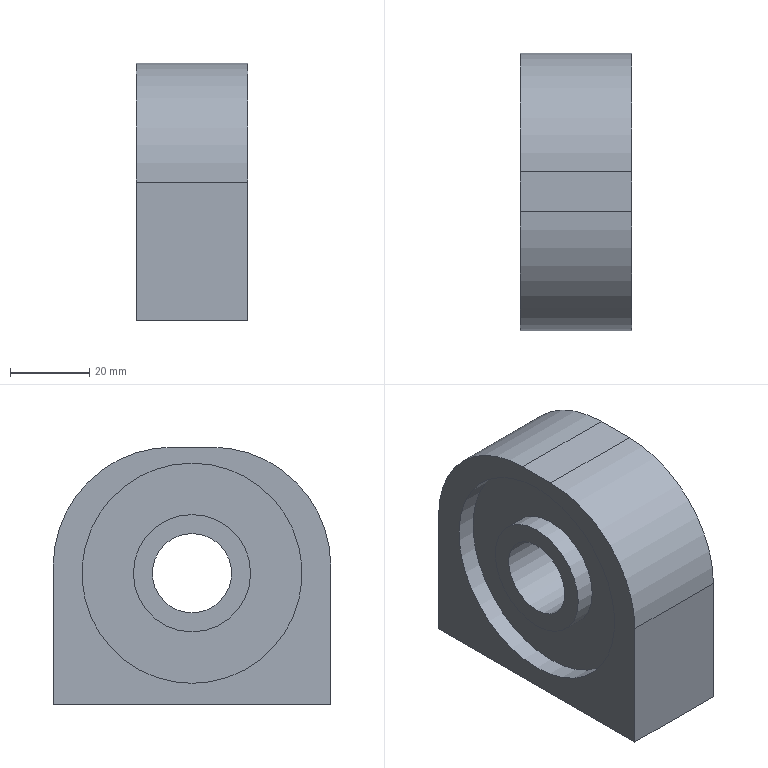Part | STEP file | Housing | 1 solid | 21 faces | box 28 x 70 x 65 mm | volume 87955 mm3 | plane 12 | cylinder 9 | commonest cylinder face diameters 8 x2 29.588 x2 55.503 x2 60 x2 20 x1
STEP:
#1=CARTESIAN_POINT('',(0.,0.,0.));
#2=DIRECTION('',(0.,0.,1.));
#3=DIRECTION('',(1.,0.,0.));
#4=AXIS2_PLACEMENT_3D('',#1,#2,#3);
#5=CARTESIAN_POINT('',(5.,-35.,47.994));
#6=VERTEX_POINT('',#5);
#7=CARTESIAN_POINT('',(5.,-35.,33.2));
#8=DIRECTION('',(-1.,0.,0.));
#9=DIRECTION('',(0.,0.,-1.));
#10=AXIS2_PLACEMENT_3D('',#7,#8,#9);
#11=CIRCLE('',#10,14.794);
#12=CARTESIAN_POINT('',(0.,-35.,33.2));
#13=DIRECTION('',(1.,0.,0.));
#14=DIRECTION('',(0.,0.,-1.));
#15=AXIS2_PLACEMENT_3D('',#12,#13,#14);
#16=CYLINDRICAL_SURFACE('',#15,14.794);
#17=CARTESIAN_POINT('',(12.566,5.));
#18=DIRECTION('',(-1.,0.));
#19=VECTOR('',#18,1.);
#20=LINE('',#17,#19);
#21=(GEOMETRIC_REPRESENTATION_CONTEXT(2)PARAMETRIC_REPRESENTATION_CONTEXT()REPRESENTATION_CONTEXT('',''));
#22=DEFINITIONAL_REPRESENTATION('',(#20),#21);
#23=PCURVE('',#16,#22);
#24=CARTESIAN_POINT('',(5.,-35.,33.2));
#25=DIRECTION('',(-1.,0.,0.));
#26=DIRECTION('',(0.,0.,1.));
#27=AXIS2_PLACEMENT_3D('',#24,#25,#26);
#28=PLANE('',#27);
#29=CARTESIAN_POINT('',(0.,0.));
#30=DIRECTION('',(-1.,0.));
#31=AXIS2_PLACEMENT_2D('',#29,#30);
#32=CIRCLE('',#31,14.794);
#33=(GEOMETRIC_REPRESENTATION_CONTEXT(2)PARAMETRIC_REPRESENTATION_CONTEXT()REPRESENTATION_CONTEXT('',''));
#34=DEFINITIONAL_REPRESENTATION('',(#32),#33);
#35=PCURVE('',#28,#34);
#36=SURFACE_CURVE('',#11,(#23,#35),.PCURVE_S1.);
#37=EDGE_CURVE('',#6,#6,#36,.T.);
#38=ORIENTED_EDGE('',*,*,#37,.T.);
#39=CARTESIAN_POINT('',(0.,-35.,47.994));
#40=VERTEX_POINT('',#39);
#41=CARTESIAN_POINT('',(0.,-35.,47.994));
#42=CARTESIAN_POINT('',(5.,-35.,47.994));
#43=B_SPLINE_CURVE_WITH_KNOTS('',1,(#41,#42),.UNSPECIFIED.,.F.,.F.,(2,2),(0.,5.),.PIECEWISE_BEZIER_KNOTS.);
#44=CARTESIAN_POINT('',(3.142,0.));
#45=DIRECTION('',(0.,1.));
#46=VECTOR('',#45,1.);
#47=LINE('',#44,#46);
#48=(GEOMETRIC_REPRESENTATION_CONTEXT(2)PARAMETRIC_REPRESENTATION_CONTEXT()REPRESENTATION_CONTEXT('',''));
#49=DEFINITIONAL_REPRESENTATION('',(#47),#48);
#50=PCURVE('',#16,#49);
#51=CARTESIAN_POINT('',(9.425,0.));
#52=DIRECTION('',(0.,1.));
#53=VECTOR('',#52,1.);
#54=LINE('',#51,#53);
#55=(GEOMETRIC_REPRESENTATION_CONTEXT(2)PARAMETRIC_REPRESENTATION_CONTEXT()REPRESENTATION_CONTEXT('',''));
#56=DEFINITIONAL_REPRESENTATION('',(#54),#55);
#57=PCURVE('',#16,#56);
#58=SEAM_CURVE('',#43,(#50,#57),.PCURVE_S1.);
#59=EDGE_CURVE('',#40,#6,#58,.T.);
#60=ORIENTED_EDGE('',*,*,#59,.F.);
#61=CARTESIAN_POINT('',(0.,-35.,33.2));
#62=DIRECTION('',(-1.,0.,0.));
#63=DIRECTION('',(0.,0.,-1.));
#64=AXIS2_PLACEMENT_3D('',#61,#62,#63);
#65=CIRCLE('',#64,14.794);
#66=CARTESIAN_POINT('',(12.566,0.));
#67=DIRECTION('',(-1.,0.));
#68=VECTOR('',#67,1.);
#69=LINE('',#66,#68);
#70=(GEOMETRIC_REPRESENTATION_CONTEXT(2)PARAMETRIC_REPRESENTATION_CONTEXT()REPRESENTATION_CONTEXT('',''));
#71=DEFINITIONAL_REPRESENTATION('',(#69),#70);
#72=PCURVE('',#16,#71);
#73=CARTESIAN_POINT('',(0.,0.,0.));
#74=DIRECTION('',(-1.,0.,0.));
#75=DIRECTION('',(0.,-1.,0.));
#76=AXIS2_PLACEMENT_3D('',#73,#74,#75);
#77=PLANE('',#76);
#78=CARTESIAN_POINT('',(35.,33.2));
#79=DIRECTION('',(0.,-1.));
#80=AXIS2_PLACEMENT_2D('',#78,#79);
#81=CIRCLE('',#80,14.794);
#82=(GEOMETRIC_REPRESENTATION_CONTEXT(2)PARAMETRIC_REPRESENTATION_CONTEXT()REPRESENTATION_CONTEXT('',''));
#83=DEFINITIONAL_REPRESENTATION('',(#81),#82);
#84=PCURVE('',#77,#83);
#85=SURFACE_CURVE('',#65,(#72,#84),.PCURVE_S1.);
#86=EDGE_CURVE('',#40,#40,#85,.T.);
#87=ORIENTED_EDGE('',*,*,#86,.F.);
#88=ORIENTED_EDGE('',*,*,#59,.T.);
#89=EDGE_LOOP('',(#38,#60,#87,#88));
#90=FACE_BOUND('',#89,.T.);
#91=ADVANCED_FACE('',(#90),#16,.T.);
#92=CARTESIAN_POINT('',(5.,-35.,60.951));
#93=VERTEX_POINT('',#92);
#94=CARTESIAN_POINT('',(5.,-35.,33.2));
#95=DIRECTION('',(1.,0.,0.));
#96=DIRECTION('',(0.,0.,-1.));
#97=AXIS2_PLACEMENT_3D('',#94,#95,#96);
#98=CIRCLE('',#97,27.751);
#99=CARTESIAN_POINT('',(0.,-35.,33.2));
#100=DIRECTION('',(1.,0.,0.));
#101=DIRECTION('',(0.,0.,-1.));
#102=AXIS2_PLACEMENT_3D('',#99,#100,#101);
#103=CYLINDRICAL_SURFACE('',#102,27.751);
#104=CARTESIAN_POINT('',(0.,5.));
#105=DIRECTION('',(1.,0.));
#106=VECTOR('',#105,1.);
#107=LINE('',#104,#106);
#108=(GEOMETRIC_REPRESENTATION_CONTEXT(2)PARAMETRIC_REPRESENTATION_CONTEXT()REPRESENTATION_CONTEXT('',''));
#109=DEFINITIONAL_REPRESENTATION('',(#107),#108);
#110=PCURVE('',#103,#109);
#111=CARTESIAN_POINT('',(-27.751,0.));
#112=CARTESIAN_POINT('',(-27.751,48.067));
#113=CARTESIAN_POINT('',(13.876,24.033));
#114=CARTESIAN_POINT('',(55.503,0.));
#115=CARTESIAN_POINT('',(13.876,-24.033));
#116=CARTESIAN_POINT('',(-27.751,-48.067));
#117=CARTESIAN_POINT('',(-27.751,0.));
#118=(BOUNDED_CURVE()B_SPLINE_CURVE(2,(#111,#112,#113,#114,#115,#116,#117),.UNSPECIFIED.,.T.,.F.)B_SPLINE_CURVE_WITH_KNOTS((1,2,2,2,2,1),(-2.094,0.,2.094,4.189,6.283,8.378),.UNSPECIFIED.)CURVE()GEOMETRIC_REPRESENTATION_ITEM()RATIONAL_B_SPLINE_CURVE((1.,0.5,1.,0.5,1.,0.5,1.))REPRESENTATION_ITEM(''));
#119=(GEOMETRIC_REPRESENTATION_CONTEXT(2)PARAMETRIC_REPRESENTATION_CONTEXT()REPRESENTATION_CONTEXT('',''));
#120=DEFINITIONAL_REPRESENTATION('',(#118),#119);
#121=PCURVE('',#28,#120);
#122=SURFACE_CURVE('',#98,(#110,#121),.PCURVE_S1.);
#123=EDGE_CURVE('',#93,#93,#122,.T.);
#124=ORIENTED_EDGE('',*,*,#123,.F.);
#125=CARTESIAN_POINT('',(0.,-35.,60.951));
#126=VERTEX_POINT('',#125);
#127=CARTESIAN_POINT('',(0.,-35.,60.951));
#128=CARTESIAN_POINT('',(5.,-35.,60.951));
#129=B_SPLINE_CURVE_WITH_KNOTS('',1,(#127,#128),.UNSPECIFIED.,.F.,.F.,(2,2),(0.,5.),.PIECEWISE_BEZIER_KNOTS.);
#130=CARTESIAN_POINT('',(3.142,0.));
#131=DIRECTION('',(0.,1.));
#132=VECTOR('',#131,1.);
#133=LINE('',#130,#132);
#134=(GEOMETRIC_REPRESENTATION_CONTEXT(2)PARAMETRIC_REPRESENTATION_CONTEXT()REPRESENTATION_CONTEXT('',''));
#135=DEFINITIONAL_REPRESENTATION('',(#133),#134);
#136=PCURVE('',#103,#135);
#137=CARTESIAN_POINT('',(9.425,0.));
#138=DIRECTION('',(0.,1.));
#139=VECTOR('',#138,1.);
#140=LINE('',#137,#139);
#141=(GEOMETRIC_REPRESENTATION_CONTEXT(2)PARAMETRIC_REPRESENTATION_CONTEXT()REPRESENTATION_CONTEXT('',''));
#142=DEFINITIONAL_REPRESENTATION('',(#140),#141);
#143=PCURVE('',#103,#142);
#144=SEAM_CURVE('',#129,(#136,#143),.PCURVE_S1.);
#145=EDGE_CURVE('',#126,#93,#144,.T.);
#146=ORIENTED_EDGE('',*,*,#145,.F.);
#147=CARTESIAN_POINT('',(0.,-35.,33.2));
#148=DIRECTION('',(1.,0.,0.));
#149=DIRECTION('',(0.,0.,-1.));
#150=AXIS2_PLACEMENT_3D('',#147,#148,#149);
#151=CIRCLE('',#150,27.751);
#152=CARTESIAN_POINT('',(0.,0.));
#153=DIRECTION('',(1.,0.));
#154=VECTOR('',#153,1.);
#155=LINE('',#152,#154);
#156=(GEOMETRIC_REPRESENTATION_CONTEXT(2)PARAMETRIC_REPRESENTATION_CONTEXT()REPRESENTATION_CONTEXT('',''));
#157=DEFINITIONAL_REPRESENTATION('',(#155),#156);
#158=PCURVE('',#103,#157);
#159=CARTESIAN_POINT('',(0.,0.,0.));
#160=DIRECTION('',(-1.,0.,0.));
#161=DIRECTION('',(0.,-1.,0.));
#162=AXIS2_PLACEMENT_3D('',#159,#160,#161);
#163=PLANE('',#162);
#164=CARTESIAN_POINT('',(35.,5.449));
#165=CARTESIAN_POINT('',(-13.067,5.449));
#166=CARTESIAN_POINT('',(10.967,47.076));
#167=CARTESIAN_POINT('',(35.,88.703));
#168=CARTESIAN_POINT('',(59.033,47.076));
#169=CARTESIAN_POINT('',(83.067,5.449));
#170=CARTESIAN_POINT('',(35.,5.449));
#171=(BOUNDED_CURVE()B_SPLINE_CURVE(2,(#164,#165,#166,#167,#168,#169,#170),.UNSPECIFIED.,.T.,.F.)B_SPLINE_CURVE_WITH_KNOTS((1,2,2,2,2,1),(-2.094,0.,2.094,4.189,6.283,8.378),.UNSPECIFIED.)CURVE()GEOMETRIC_REPRESENTATION_ITEM()RATIONAL_B_SPLINE_CURVE((1.,0.5,1.,0.5,1.,0.5,1.))REPRESENTATION_ITEM(''));
#172=(GEOMETRIC_REPRESENTATION_CONTEXT(2)PARAMETRIC_REPRESENTATION_CONTEXT()REPRESENTATION_CONTEXT('',''));
#173=DEFINITIONAL_REPRESENTATION('',(#171),#172);
#174=PCURVE('',#163,#173);
#175=SURFACE_CURVE('',#151,(#158,#174),.PCURVE_S1.);
#176=EDGE_CURVE('',#126,#126,#175,.T.);
#177=ORIENTED_EDGE('',*,*,#176,.T.);
#178=ORIENTED_EDGE('',*,*,#145,.T.);
#179=EDGE_LOOP('',(#124,#146,#177,#178));
#180=FACE_BOUND('',#179,.F.);
#181=ADVANCED_FACE('',(#180),#103,.F.);
#182=ORIENTED_EDGE('',*,*,#123,.F.);
#183=EDGE_LOOP('',(#182));
#184=FACE_BOUND('',#183,.T.);
#185=ORIENTED_EDGE('',*,*,#37,.F.);
#186=EDGE_LOOP('',(#185));
#187=FACE_BOUND('',#186,.T.);
#188=ADVANCED_FACE('',(#184,#187),#28,.T.);
#189=CARTESIAN_POINT('',(0.,-40.,65.));
#190=VERTEX_POINT('',#189);
#191=CARTESIAN_POINT('',(0.,-70.,35.));
#192=VERTEX_POINT('',#191);
#193=CARTESIAN_POINT('',(0.,-40.,35.));
#194=DIRECTION('',(1.,0.,0.));
#195=DIRECTION('',(0.,-0.7071,0.7071));
#196=AXIS2_PLACEMENT_3D('',#193,#194,#195);
#197=CIRCLE('',#196,30.);
#198=CARTESIAN_POINT('',(61.213,56.213));
#199=CARTESIAN_POINT('',(97.956,19.471));
#200=CARTESIAN_POINT('',(47.765,6.022));
#201=CARTESIAN_POINT('',(-2.426,-7.426));
#202=CARTESIAN_POINT('',(11.022,42.765));
#203=CARTESIAN_POINT('',(24.471,92.956));
#204=CARTESIAN_POINT('',(61.213,56.213));
#205=(BOUNDED_CURVE()B_SPLINE_CURVE(2,(#198,#199,#200,#201,#202,#203,#204),.UNSPECIFIED.,.T.,.F.)B_SPLINE_CURVE_WITH_KNOTS((1,2,2,2,2,1),(-2.094,0.,2.094,4.189,6.283,8.378),.UNSPECIFIED.)CURVE()GEOMETRIC_REPRESENTATION_ITEM()RATIONAL_B_SPLINE_CURVE((1.,0.5,1.,0.5,1.,0.5,1.))REPRESENTATION_ITEM(''));
#206=(GEOMETRIC_REPRESENTATION_CONTEXT(2)PARAMETRIC_REPRESENTATION_CONTEXT()REPRESENTATION_CONTEXT('',''));
#207=DEFINITIONAL_REPRESENTATION('',(#205),#206);
#208=PCURVE('',#163,#207);
#209=CARTESIAN_POINT('',(7.,-40.,35.));
#210=DIRECTION('',(1.,0.,0.));
#211=DIRECTION('',(0.,-0.7071,0.7071));
#212=AXIS2_PLACEMENT_3D('',#209,#210,#211);
#213=CYLINDRICAL_SURFACE('',#212,30.);
#214=CARTESIAN_POINT('',(-6.283,-7.));
#215=DIRECTION('',(1.,0.));
#216=VECTOR('',#215,1.);
#217=LINE('',#214,#216);
#218=(GEOMETRIC_REPRESENTATION_CONTEXT(2)PARAMETRIC_REPRESENTATION_CONTEXT()REPRESENTATION_CONTEXT('',''));
#219=DEFINITIONAL_REPRESENTATION('',(#217),#218);
#220=PCURVE('',#213,#219);
#221=SURFACE_CURVE('',#197,(#208,#220),.PCURVE_S1.);
#222=EDGE_CURVE('',#190,#192,#221,.T.);
#223=ORIENTED_EDGE('',*,*,#222,.F.);
#224=CARTESIAN_POINT('',(0.,-30.,65.));
#225=VERTEX_POINT('',#224);
#226=CARTESIAN_POINT('',(0.,-70.,65.));
#227=DIRECTION('',(0.,-1.,0.));
#228=VECTOR('',#227,1.);
#229=LINE('',#226,#228);
#230=CARTESIAN_POINT('',(70.,65.));
#231=DIRECTION('',(1.,0.));
#232=VECTOR('',#231,1.);
#233=LINE('',#230,#232);
#234=(GEOMETRIC_REPRESENTATION_CONTEXT(2)PARAMETRIC_REPRESENTATION_CONTEXT()REPRESENTATION_CONTEXT('',''));
#235=DEFINITIONAL_REPRESENTATION('',(#233),#234);
#236=PCURVE('',#163,#235);
#237=CARTESIAN_POINT('',(14.,-35.,65.));
#238=DIRECTION('',(0.,0.,1.));
#239=DIRECTION('',(1.,0.,0.));
#240=AXIS2_PLACEMENT_3D('',#237,#238,#239);
#241=PLANE('',#240);
#242=CARTESIAN_POINT('',(-14.,-35.));
#243=DIRECTION('',(0.,-1.));
#244=VECTOR('',#243,1.);
#245=LINE('',#242,#244);
#246=(GEOMETRIC_REPRESENTATION_CONTEXT(2)PARAMETRIC_REPRESENTATION_CONTEXT()REPRESENTATION_CONTEXT('',''));
#247=DEFINITIONAL_REPRESENTATION('',(#245),#246);
#248=PCURVE('',#241,#247);
#249=SURFACE_CURVE('',#229,(#236,#248),.PCURVE_S1.);
#250=EDGE_CURVE('',#225,#190,#249,.T.);
#251=ORIENTED_EDGE('',*,*,#250,.F.);
#252=CARTESIAN_POINT('',(0.,0.,35.));
#253=VERTEX_POINT('',#252);
#254=CARTESIAN_POINT('',(0.,-30.,35.));
#255=DIRECTION('',(1.,0.,0.));
#256=DIRECTION('',(0.,0.7071,0.7071));
#257=AXIS2_PLACEMENT_3D('',#254,#255,#256);
#258=CIRCLE('',#257,30.);
#259=CARTESIAN_POINT('',(8.787,56.213));
#260=CARTESIAN_POINT('',(45.529,92.956));
#261=CARTESIAN_POINT('',(58.978,42.765));
#262=CARTESIAN_POINT('',(72.426,-7.426));
#263=CARTESIAN_POINT('',(22.235,6.022));
#264=CARTESIAN_POINT('',(-27.956,19.471));
#265=CARTESIAN_POINT('',(8.787,56.213));
#266=(BOUNDED_CURVE()B_SPLINE_CURVE(2,(#259,#260,#261,#262,#263,#264,#265),.UNSPECIFIED.,.T.,.F.)B_SPLINE_CURVE_WITH_KNOTS((1,2,2,2,2,1),(-2.094,0.,2.094,4.189,6.283,8.378),.UNSPECIFIED.)CURVE()GEOMETRIC_REPRESENTATION_ITEM()RATIONAL_B_SPLINE_CURVE((1.,0.5,1.,0.5,1.,0.5,1.))REPRESENTATION_ITEM(''));
#267=(GEOMETRIC_REPRESENTATION_CONTEXT(2)PARAMETRIC_REPRESENTATION_CONTEXT()REPRESENTATION_CONTEXT('',''));
#268=DEFINITIONAL_REPRESENTATION('',(#266),#267);
#269=PCURVE('',#163,#268);
#270=CARTESIAN_POINT('',(21.,-30.,35.));
#271=DIRECTION('',(-1.,0.,0.));
#272=DIRECTION('',(0.,0.7071,0.7071));
#273=AXIS2_PLACEMENT_3D('',#270,#271,#272);
#274=CYLINDRICAL_SURFACE('',#273,30.);
#275=CARTESIAN_POINT('',(12.566,21.));
#276=DIRECTION('',(-1.,0.));
#277=VECTOR('',#276,1.);
#278=LINE('',#275,#277);
#279=(GEOMETRIC_REPRESENTATION_CONTEXT(2)PARAMETRIC_REPRESENTATION_CONTEXT()REPRESENTATION_CONTEXT('',''));
#280=DEFINITIONAL_REPRESENTATION('',(#278),#279);
#281=PCURVE('',#274,#280);
#282=SURFACE_CURVE('',#258,(#269,#281),.PCURVE_S1.);
#283=EDGE_CURVE('',#253,#225,#282,.T.);
#284=ORIENTED_EDGE('',*,*,#283,.F.);
#285=CARTESIAN_POINT('',(0.,0.,0.));
#286=VERTEX_POINT('',#285);
#287=CARTESIAN_POINT('',(0.,0.,0.));
#288=DIRECTION('',(0.,0.,1.));
#289=VECTOR('',#288,1.);
#290=LINE('',#287,#289);
#291=CARTESIAN_POINT('',(0.,0.));
#292=DIRECTION('',(0.,1.));
#293=VECTOR('',#292,1.);
#294=LINE('',#291,#293);
#295=(GEOMETRIC_REPRESENTATION_CONTEXT(2)PARAMETRIC_REPRESENTATION_CONTEXT()REPRESENTATION_CONTEXT('',''));
#296=DEFINITIONAL_REPRESENTATION('',(#294),#295);
#297=PCURVE('',#163,#296);
#298=CARTESIAN_POINT('',(28.,0.,0.));
#299=DIRECTION('',(0.,1.,0.));
#300=DIRECTION('',(-1.,0.,0.));
#301=AXIS2_PLACEMENT_3D('',#298,#299,#300);
#302=PLANE('',#301);
#303=CARTESIAN_POINT('',(28.,0.));
#304=DIRECTION('',(0.,1.));
#305=VECTOR('',#304,1.);
#306=LINE('',#303,#305);
#307=(GEOMETRIC_REPRESENTATION_CONTEXT(2)PARAMETRIC_REPRESENTATION_CONTEXT()REPRESENTATION_CONTEXT('',''));
#308=DEFINITIONAL_REPRESENTATION('',(#306),#307);
#309=PCURVE('',#302,#308);
#310=SURFACE_CURVE('',#290,(#297,#309),.PCURVE_S1.);
#311=EDGE_CURVE('',#286,#253,#310,.T.);
#312=ORIENTED_EDGE('',*,*,#311,.F.);
#313=CARTESIAN_POINT('',(0.,-70.,0.));
#314=VERTEX_POINT('',#313);
#315=CARTESIAN_POINT('',(0.,-70.,0.));
#316=DIRECTION('',(0.,1.,0.));
#317=VECTOR('',#316,1.);
#318=LINE('',#315,#317);
#319=CARTESIAN_POINT('',(70.,0.));
#320=DIRECTION('',(-1.,0.));
#321=VECTOR('',#320,1.);
#322=LINE('',#319,#321);
#323=(GEOMETRIC_REPRESENTATION_CONTEXT(2)PARAMETRIC_REPRESENTATION_CONTEXT()REPRESENTATION_CONTEXT('',''));
#324=DEFINITIONAL_REPRESENTATION('',(#322),#323);
#325=PCURVE('',#163,#324);
#326=CARTESIAN_POINT('',(14.,-35.,0.));
#327=DIRECTION('',(0.,0.,1.));
#328=DIRECTION('',(1.,0.,0.));
#329=AXIS2_PLACEMENT_3D('',#326,#327,#328);
#330=PLANE('',#329);
#331=CARTESIAN_POINT('',(-14.,-35.));
#332=DIRECTION('',(0.,1.));
#333=VECTOR('',#332,1.);
#334=LINE('',#331,#333);
#335=(GEOMETRIC_REPRESENTATION_CONTEXT(2)PARAMETRIC_REPRESENTATION_CONTEXT()REPRESENTATION_CONTEXT('',''));
#336=DEFINITIONAL_REPRESENTATION('',(#334),#335);
#337=PCURVE('',#330,#336);
#338=SURFACE_CURVE('',#318,(#325,#337),.PCURVE_S1.);
#339=EDGE_CURVE('',#314,#286,#338,.T.);
#340=ORIENTED_EDGE('',*,*,#339,.F.);
#341=CARTESIAN_POINT('',(0.,-70.,0.));
#342=DIRECTION('',(0.,0.,1.));
#343=VECTOR('',#342,1.);
#344=LINE('',#341,#343);
#345=CARTESIAN_POINT('',(70.,0.));
#346=DIRECTION('',(0.,1.));
#347=VECTOR('',#346,1.);
#348=LINE('',#345,#347);
#349=(GEOMETRIC_REPRESENTATION_CONTEXT(2)PARAMETRIC_REPRESENTATION_CONTEXT()REPRESENTATION_CONTEXT('',''));
#350=DEFINITIONAL_REPRESENTATION('',(#348),#349);
#351=PCURVE('',#163,#350);
#352=CARTESIAN_POINT('',(0.,-70.,0.));
#353=DIRECTION('',(0.,-1.,0.));
#354=DIRECTION('',(1.,0.,0.));
#355=AXIS2_PLACEMENT_3D('',#352,#353,#354);
#356=PLANE('',#355);
#357=CARTESIAN_POINT('',(0.,0.));
#358=DIRECTION('',(0.,1.));
#359=VECTOR('',#358,1.);
#360=LINE('',#357,#359);
#361=(GEOMETRIC_REPRESENTATION_CONTEXT(2)PARAMETRIC_REPRESENTATION_CONTEXT()REPRESENTATION_CONTEXT('',''));
#362=DEFINITIONAL_REPRESENTATION('',(#360),#361);
#363=PCURVE('',#356,#362);
#364=SURFACE_CURVE('',#344,(#351,#363),.PCURVE_S1.);
#365=EDGE_CURVE('',#314,#192,#364,.T.);
#366=ORIENTED_EDGE('',*,*,#365,.T.);
#367=EDGE_LOOP('',(#223,#251,#284,#312,#340,#366));
#368=FACE_BOUND('',#367,.T.);
#369=ORIENTED_EDGE('',*,*,#176,.T.);
#370=EDGE_LOOP('',(#369));
#371=FACE_BOUND('',#370,.T.);
#372=ADVANCED_FACE('',(#368,#371),#163,.T.);
#373=CARTESIAN_POINT('',(23.,-35.,18.406));
#374=VERTEX_POINT('',#373);
#375=CARTESIAN_POINT('',(23.,-35.,33.2));
#376=DIRECTION('',(1.,0.,0.));
#377=DIRECTION('',(0.,0.,1.));
#378=AXIS2_PLACEMENT_3D('',#375,#376,#377);
#379=CIRCLE('',#378,14.794);
#380=CARTESIAN_POINT('',(28.,-35.,33.2));
#381=DIRECTION('',(-1.,0.,0.));
#382=DIRECTION('',(0.,0.,1.));
#383=AXIS2_PLACEMENT_3D('',#380,#381,#382);
#384=CYLINDRICAL_SURFACE('',#383,14.794);
#385=CARTESIAN_POINT('',(12.566,5.));
#386=DIRECTION('',(-1.,0.));
#387=VECTOR('',#386,1.);
#388=LINE('',#385,#387);
#389=(GEOMETRIC_REPRESENTATION_CONTEXT(2)PARAMETRIC_REPRESENTATION_CONTEXT()REPRESENTATION_CONTEXT('',''));
#390=DEFINITIONAL_REPRESENTATION('',(#388),#389);
#391=PCURVE('',#384,#390);
#392=CARTESIAN_POINT('',(23.,-35.,33.2));
#393=DIRECTION('',(-1.,0.,0.));
#394=DIRECTION('',(0.,0.,1.));
#395=AXIS2_PLACEMENT_3D('',#392,#393,#394);
#396=PLANE('',#395);
#397=CARTESIAN_POINT('',(14.794,0.));
#398=CARTESIAN_POINT('',(14.794,-25.624));
#399=CARTESIAN_POINT('',(-7.397,-12.812));
#400=CARTESIAN_POINT('',(-29.588,0.));
#401=CARTESIAN_POINT('',(-7.397,12.812));
#402=CARTESIAN_POINT('',(14.794,25.624));
#403=CARTESIAN_POINT('',(14.794,0.));
#404=(BOUNDED_CURVE()B_SPLINE_CURVE(2,(#397,#398,#399,#400,#401,#402,#403),.UNSPECIFIED.,.T.,.F.)B_SPLINE_CURVE_WITH_KNOTS((1,2,2,2,2,1),(-2.094,0.,2.094,4.189,6.283,8.378),.UNSPECIFIED.)CURVE()GEOMETRIC_REPRESENTATION_ITEM()RATIONAL_B_SPLINE_CURVE((1.,0.5,1.,0.5,1.,0.5,1.))REPRESENTATION_ITEM(''));
#405=(GEOMETRIC_REPRESENTATION_CONTEXT(2)PARAMETRIC_REPRESENTATION_CONTEXT()REPRESENTATION_CONTEXT('',''));
#406=DEFINITIONAL_REPRESENTATION('',(#404),#405);
#407=PCURVE('',#396,#406);
#408=SURFACE_CURVE('',#379,(#391,#407),.PCURVE_S1.);
#409=EDGE_CURVE('',#374,#374,#408,.T.);
#410=ORIENTED_EDGE('',*,*,#409,.T.);
#411=CARTESIAN_POINT('',(28.,-35.,18.406));
#412=VERTEX_POINT('',#411);
#413=CARTESIAN_POINT('',(28.,-35.,18.406));
#414=CARTESIAN_POINT('',(23.,-35.,18.406));
#415=B_SPLINE_CURVE_WITH_KNOTS('',1,(#413,#414),.UNSPECIFIED.,.F.,.F.,(2,2),(0.,5.),.PIECEWISE_BEZIER_KNOTS.);
#416=CARTESIAN_POINT('',(3.142,0.));
#417=DIRECTION('',(0.,1.));
#418=VECTOR('',#417,1.);
#419=LINE('',#416,#418);
#420=(GEOMETRIC_REPRESENTATION_CONTEXT(2)PARAMETRIC_REPRESENTATION_CONTEXT()REPRESENTATION_CONTEXT('',''));
#421=DEFINITIONAL_REPRESENTATION('',(#419),#420);
#422=PCURVE('',#384,#421);
#423=CARTESIAN_POINT('',(9.425,0.));
#424=DIRECTION('',(0.,1.));
#425=VECTOR('',#424,1.);
#426=LINE('',#423,#425);
#427=(GEOMETRIC_REPRESENTATION_CONTEXT(2)PARAMETRIC_REPRESENTATION_CONTEXT()REPRESENTATION_CONTEXT('',''));
#428=DEFINITIONAL_REPRESENTATION('',(#426),#427);
#429=PCURVE('',#384,#428);
#430=SEAM_CURVE('',#415,(#422,#429),.PCURVE_S1.);
#431=EDGE_CURVE('',#412,#374,#430,.T.);
#432=ORIENTED_EDGE('',*,*,#431,.F.);
#433=CARTESIAN_POINT('',(28.,-35.,33.2));
#434=DIRECTION('',(1.,0.,0.));
#435=DIRECTION('',(0.,0.,1.));
#436=AXIS2_PLACEMENT_3D('',#433,#434,#435);
#437=CIRCLE('',#436,14.794);
#438=CARTESIAN_POINT('',(12.566,0.));
#439=DIRECTION('',(-1.,0.));
#440=VECTOR('',#439,1.);
#441=LINE('',#438,#440);
#442=(GEOMETRIC_REPRESENTATION_CONTEXT(2)PARAMETRIC_REPRESENTATION_CONTEXT()REPRESENTATION_CONTEXT('',''));
#443=DEFINITIONAL_REPRESENTATION('',(#441),#442);
#444=PCURVE('',#384,#443);
#445=CARTESIAN_POINT('',(28.,-70.,0.));
#446=DIRECTION('',(1.,0.,0.));
#447=DIRECTION('',(0.,1.,0.));
#448=AXIS2_PLACEMENT_3D('',#445,#446,#447);
#449=PLANE('',#448);
#450=CARTESIAN_POINT('',(35.,33.2));
#451=DIRECTION('',(0.,1.));
#452=AXIS2_PLACEMENT_2D('',#450,#451);
#453=CIRCLE('',#452,14.794);
#454=(GEOMETRIC_REPRESENTATION_CONTEXT(2)PARAMETRIC_REPRESENTATION_CONTEXT()REPRESENTATION_CONTEXT('',''));
#455=DEFINITIONAL_REPRESENTATION('',(#453),#454);
#456=PCURVE('',#449,#455);
#457=SURFACE_CURVE('',#437,(#444,#456),.PCURVE_S1.);
#458=EDGE_CURVE('',#412,#412,#457,.T.);
#459=ORIENTED_EDGE('',*,*,#458,.F.);
#460=ORIENTED_EDGE('',*,*,#431,.T.);
#461=EDGE_LOOP('',(#410,#432,#459,#460));
#462=FACE_BOUND('',#461,.T.);
#463=ADVANCED_FACE('',(#462),#384,.T.);
#464=CARTESIAN_POINT('',(23.,-35.,5.449));
#465=VERTEX_POINT('',#464);
#466=CARTESIAN_POINT('',(23.,-35.,33.2));
#467=DIRECTION('',(-1.,0.,0.));
#468=DIRECTION('',(0.,0.,1.));
#469=AXIS2_PLACEMENT_3D('',#466,#467,#468);
#470=CIRCLE('',#469,27.751);
#471=CARTESIAN_POINT('',(28.,-35.,33.2));
#472=DIRECTION('',(-1.,0.,0.));
#473=DIRECTION('',(0.,0.,1.));
#474=AXIS2_PLACEMENT_3D('',#471,#472,#473);
#475=CYLINDRICAL_SURFACE('',#474,27.751);
#476=CARTESIAN_POINT('',(0.,5.));
#477=DIRECTION('',(1.,0.));
#478=VECTOR('',#477,1.);
#479=LINE('',#476,#478);
#480=(GEOMETRIC_REPRESENTATION_CONTEXT(2)PARAMETRIC_REPRESENTATION_CONTEXT()REPRESENTATION_CONTEXT('',''));
#481=DEFINITIONAL_REPRESENTATION('',(#479),#480);
#482=PCURVE('',#475,#481);
#483=CARTESIAN_POINT('',(0.,0.));
#484=DIRECTION('',(1.,0.));
#485=AXIS2_PLACEMENT_2D('',#483,#484);
#486=CIRCLE('',#485,27.751);
#487=(GEOMETRIC_REPRESENTATION_CONTEXT(2)PARAMETRIC_REPRESENTATION_CONTEXT()REPRESENTATION_CONTEXT('',''));
#488=DEFINITIONAL_REPRESENTATION('',(#486),#487);
#489=PCURVE('',#396,#488);
#490=SURFACE_CURVE('',#470,(#482,#489),.PCURVE_S1.);
#491=EDGE_CURVE('',#465,#465,#490,.T.);
#492=ORIENTED_EDGE('',*,*,#491,.F.);
#493=CARTESIAN_POINT('',(28.,-35.,5.449));
#494=VERTEX_POINT('',#493);
#495=CARTESIAN_POINT('',(28.,-35.,5.449));
#496=CARTESIAN_POINT('',(23.,-35.,5.449));
#497=B_SPLINE_CURVE_WITH_KNOTS('',1,(#495,#496),.UNSPECIFIED.,.F.,.F.,(2,2),(0.,5.),.PIECEWISE_BEZIER_KNOTS.);
#498=CARTESIAN_POINT('',(3.142,0.));
#499=DIRECTION('',(0.,1.));
#500=VECTOR('',#499,1.);
#501=LINE('',#498,#500);
#502=(GEOMETRIC_REPRESENTATION_CONTEXT(2)PARAMETRIC_REPRESENTATION_CONTEXT()REPRESENTATION_CONTEXT('',''));
#503=DEFINITIONAL_REPRESENTATION('',(#501),#502);
#504=PCURVE('',#475,#503);
#505=CARTESIAN_POINT('',(9.425,0.));
#506=DIRECTION('',(0.,1.));
#507=VECTOR('',#506,1.);
#508=LINE('',#505,#507);
#509=(GEOMETRIC_REPRESENTATION_CONTEXT(2)PARAMETRIC_REPRESENTATION_CONTEXT()REPRESENTATION_CONTEXT('',''));
#510=DEFINITIONAL_REPRESENTATION('',(#508),#509);
#511=PCURVE('',#475,#510);
#512=SEAM_CURVE('',#497,(#504,#511),.PCURVE_S1.);
#513=EDGE_CURVE('',#494,#465,#512,.T.);
#514=ORIENTED_EDGE('',*,*,#513,.F.);
#515=CARTESIAN_POINT('',(28.,-35.,33.2));
#516=DIRECTION('',(-1.,0.,0.));
#517=DIRECTION('',(0.,0.,1.));
#518=AXIS2_PLACEMENT_3D('',#515,#516,#517);
#519=CIRCLE('',#518,27.751);
#520=CARTESIAN_POINT('',(0.,0.));
#521=DIRECTION('',(1.,0.));
#522=VECTOR('',#521,1.);
#523=LINE('',#520,#522);
#524=(GEOMETRIC_REPRESENTATION_CONTEXT(2)PARAMETRIC_REPRESENTATION_CONTEXT()REPRESENTATION_CONTEXT('',''));
#525=DEFINITIONAL_REPRESENTATION('',(#523),#524);
#526=PCURVE('',#475,#525);
#527=CARTESIAN_POINT('',(28.,-70.,0.));
#528=DIRECTION('',(1.,0.,0.));
#529=DIRECTION('',(0.,1.,0.));
#530=AXIS2_PLACEMENT_3D('',#527,#528,#529);
#531=PLANE('',#530);
#532=CARTESIAN_POINT('',(35.,60.951));
#533=CARTESIAN_POINT('',(83.067,60.951));
#534=CARTESIAN_POINT('',(59.033,19.324));
#535=CARTESIAN_POINT('',(35.,-22.303));
#536=CARTESIAN_POINT('',(10.967,19.324));
#537=CARTESIAN_POINT('',(-13.067,60.951));
#538=CARTESIAN_POINT('',(35.,60.951));
#539=(BOUNDED_CURVE()B_SPLINE_CURVE(2,(#532,#533,#534,#535,#536,#537,#538),.UNSPECIFIED.,.T.,.F.)B_SPLINE_CURVE_WITH_KNOTS((1,2,2,2,2,1),(-2.094,0.,2.094,4.189,6.283,8.378),.UNSPECIFIED.)CURVE()GEOMETRIC_REPRESENTATION_ITEM()RATIONAL_B_SPLINE_CURVE((1.,0.5,1.,0.5,1.,0.5,1.))REPRESENTATION_ITEM(''));
#540=(GEOMETRIC_REPRESENTATION_CONTEXT(2)PARAMETRIC_REPRESENTATION_CONTEXT()REPRESENTATION_CONTEXT('',''));
#541=DEFINITIONAL_REPRESENTATION('',(#539),#540);
#542=PCURVE('',#531,#541);
#543=SURFACE_CURVE('',#519,(#526,#542),.PCURVE_S1.);
#544=EDGE_CURVE('',#494,#494,#543,.T.);
#545=ORIENTED_EDGE('',*,*,#544,.T.);
#546=ORIENTED_EDGE('',*,*,#513,.T.);
#547=EDGE_LOOP('',(#492,#514,#545,#546));
#548=FACE_BOUND('',#547,.F.);
#549=ADVANCED_FACE('',(#548),#475,.F.);
#550=ORIENTED_EDGE('',*,*,#491,.F.);
#551=EDGE_LOOP('',(#550));
#552=FACE_BOUND('',#551,.T.);
#553=ORIENTED_EDGE('',*,*,#409,.F.);
#554=EDGE_LOOP('',(#553));
#555=FACE_BOUND('',#554,.T.);
#556=ADVANCED_FACE('',(#552,#555),#396,.F.);
#557=CARTESIAN_POINT('',(28.,-70.,35.));
#558=VERTEX_POINT('',#557);
#559=CARTESIAN_POINT('',(28.,-40.,65.));
#560=VERTEX_POINT('',#559);
#561=CARTESIAN_POINT('',(28.,-40.,35.));
#562=DIRECTION('',(-1.,0.,0.));
#563=DIRECTION('',(0.,-0.7071,0.7071));
#564=AXIS2_PLACEMENT_3D('',#561,#562,#563);
#565=CIRCLE('',#564,30.);
#566=CARTESIAN_POINT('',(8.787,56.213));
#567=CARTESIAN_POINT('',(45.529,92.956));
#568=CARTESIAN_POINT('',(58.978,42.765));
#569=CARTESIAN_POINT('',(72.426,-7.426));
#570=CARTESIAN_POINT('',(22.235,6.022));
#571=CARTESIAN_POINT('',(-27.956,19.471));
#572=CARTESIAN_POINT('',(8.787,56.213));
#573=(BOUNDED_CURVE()B_SPLINE_CURVE(2,(#566,#567,#568,#569,#570,#571,#572),.UNSPECIFIED.,.T.,.F.)B_SPLINE_CURVE_WITH_KNOTS((1,2,2,2,2,1),(-2.094,0.,2.094,4.189,6.283,8.378),.UNSPECIFIED.)CURVE()GEOMETRIC_REPRESENTATION_ITEM()RATIONAL_B_SPLINE_CURVE((1.,0.5,1.,0.5,1.,0.5,1.))REPRESENTATION_ITEM(''));
#574=(GEOMETRIC_REPRESENTATION_CONTEXT(2)PARAMETRIC_REPRESENTATION_CONTEXT()REPRESENTATION_CONTEXT('',''));
#575=DEFINITIONAL_REPRESENTATION('',(#573),#574);
#576=PCURVE('',#531,#575);
#577=CARTESIAN_POINT('',(6.283,21.));
#578=DIRECTION('',(-1.,0.));
#579=VECTOR('',#578,1.);
#580=LINE('',#577,#579);
#581=(GEOMETRIC_REPRESENTATION_CONTEXT(2)PARAMETRIC_REPRESENTATION_CONTEXT()REPRESENTATION_CONTEXT('',''));
#582=DEFINITIONAL_REPRESENTATION('',(#580),#581);
#583=PCURVE('',#213,#582);
#584=SURFACE_CURVE('',#565,(#576,#583),.PCURVE_S1.);
#585=EDGE_CURVE('',#558,#560,#584,.T.);
#586=ORIENTED_EDGE('',*,*,#585,.F.);
#587=CARTESIAN_POINT('',(28.,-70.,0.));
#588=VERTEX_POINT('',#587);
#589=CARTESIAN_POINT('',(28.,-70.,0.));
#590=DIRECTION('',(0.,0.,1.));
#591=VECTOR('',#590,1.);
#592=LINE('',#589,#591);
#593=CARTESIAN_POINT('',(0.,0.));
#594=DIRECTION('',(0.,1.));
#595=VECTOR('',#594,1.);
#596=LINE('',#593,#595);
#597=(GEOMETRIC_REPRESENTATION_CONTEXT(2)PARAMETRIC_REPRESENTATION_CONTEXT()REPRESENTATION_CONTEXT('',''));
#598=DEFINITIONAL_REPRESENTATION('',(#596),#597);
#599=PCURVE('',#531,#598);
#600=CARTESIAN_POINT('',(28.,0.));
#601=DIRECTION('',(0.,1.));
#602=VECTOR('',#601,1.);
#603=LINE('',#600,#602);
#604=(GEOMETRIC_REPRESENTATION_CONTEXT(2)PARAMETRIC_REPRESENTATION_CONTEXT()REPRESENTATION_CONTEXT('',''));
#605=DEFINITIONAL_REPRESENTATION('',(#603),#604);
#606=PCURVE('',#356,#605);
#607=SURFACE_CURVE('',#592,(#599,#606),.PCURVE_S1.);
#608=EDGE_CURVE('',#588,#558,#607,.T.);
#609=ORIENTED_EDGE('',*,*,#608,.F.);
#610=CARTESIAN_POINT('',(28.,0.,0.));
#611=VERTEX_POINT('',#610);
#612=CARTESIAN_POINT('',(28.,0.,0.));
#613=DIRECTION('',(0.,-1.,0.));
#614=VECTOR('',#613,1.);
#615=LINE('',#612,#614);
#616=CARTESIAN_POINT('',(70.,0.));
#617=DIRECTION('',(-1.,0.));
#618=VECTOR('',#617,1.);
#619=LINE('',#616,#618);
#620=(GEOMETRIC_REPRESENTATION_CONTEXT(2)PARAMETRIC_REPRESENTATION_CONTEXT()REPRESENTATION_CONTEXT('',''));
#621=DEFINITIONAL_REPRESENTATION('',(#619),#620);
#622=PCURVE('',#531,#621);
#623=CARTESIAN_POINT('',(14.,35.));
#624=DIRECTION('',(0.,-1.));
#625=VECTOR('',#624,1.);
#626=LINE('',#623,#625);
#627=(GEOMETRIC_REPRESENTATION_CONTEXT(2)PARAMETRIC_REPRESENTATION_CONTEXT()REPRESENTATION_CONTEXT('',''));
#628=DEFINITIONAL_REPRESENTATION('',(#626),#627);
#629=PCURVE('',#330,#628);
#630=SURFACE_CURVE('',#615,(#622,#629),.PCURVE_S1.);
#631=EDGE_CURVE('',#611,#588,#630,.T.);
#632=ORIENTED_EDGE('',*,*,#631,.F.);
#633=CARTESIAN_POINT('',(28.,0.,35.));
#634=VERTEX_POINT('',#633);
#635=CARTESIAN_POINT('',(28.,0.,0.));
#636=DIRECTION('',(0.,0.,1.));
#637=VECTOR('',#636,1.);
#638=LINE('',#635,#637);
#639=CARTESIAN_POINT('',(70.,0.));
#640=DIRECTION('',(0.,1.));
#641=VECTOR('',#640,1.);
#642=LINE('',#639,#641);
#643=(GEOMETRIC_REPRESENTATION_CONTEXT(2)PARAMETRIC_REPRESENTATION_CONTEXT()REPRESENTATION_CONTEXT('',''));
#644=DEFINITIONAL_REPRESENTATION('',(#642),#643);
#645=PCURVE('',#531,#644);
#646=CARTESIAN_POINT('',(0.,0.));
#647=DIRECTION('',(0.,1.));
#648=VECTOR('',#647,1.);
#649=LINE('',#646,#648);
#650=(GEOMETRIC_REPRESENTATION_CONTEXT(2)PARAMETRIC_REPRESENTATION_CONTEXT()REPRESENTATION_CONTEXT('',''));
#651=DEFINITIONAL_REPRESENTATION('',(#649),#650);
#652=PCURVE('',#302,#651);
#653=SURFACE_CURVE('',#638,(#645,#652),.PCURVE_S1.);
#654=EDGE_CURVE('',#611,#634,#653,.T.);
#655=ORIENTED_EDGE('',*,*,#654,.T.);
#656=CARTESIAN_POINT('',(28.,-30.,65.));
#657=VERTEX_POINT('',#656);
#658=CARTESIAN_POINT('',(28.,-30.,35.));
#659=DIRECTION('',(-1.,0.,0.));
#660=DIRECTION('',(0.,0.7071,0.7071));
#661=AXIS2_PLACEMENT_3D('',#658,#659,#660);
#662=CIRCLE('',#661,30.);
#663=CARTESIAN_POINT('',(61.213,56.213));
#664=CARTESIAN_POINT('',(97.956,19.471));
#665=CARTESIAN_POINT('',(47.765,6.022));
#666=CARTESIAN_POINT('',(-2.426,-7.426));
#667=CARTESIAN_POINT('',(11.022,42.765));
#668=CARTESIAN_POINT('',(24.471,92.956));
#669=CARTESIAN_POINT('',(61.213,56.213));
#670=(BOUNDED_CURVE()B_SPLINE_CURVE(2,(#663,#664,#665,#666,#667,#668,#669),.UNSPECIFIED.,.T.,.F.)B_SPLINE_CURVE_WITH_KNOTS((1,2,2,2,2,1),(-2.094,0.,2.094,4.189,6.283,8.378),.UNSPECIFIED.)CURVE()GEOMETRIC_REPRESENTATION_ITEM()RATIONAL_B_SPLINE_CURVE((1.,0.5,1.,0.5,1.,0.5,1.))REPRESENTATION_ITEM(''));
#671=(GEOMETRIC_REPRESENTATION_CONTEXT(2)PARAMETRIC_REPRESENTATION_CONTEXT()REPRESENTATION_CONTEXT('',''));
#672=DEFINITIONAL_REPRESENTATION('',(#670),#671);
#673=PCURVE('',#531,#672);
#674=CARTESIAN_POINT('',(0.,-7.));
#675=DIRECTION('',(1.,0.));
#676=VECTOR('',#675,1.);
#677=LINE('',#674,#676);
#678=(GEOMETRIC_REPRESENTATION_CONTEXT(2)PARAMETRIC_REPRESENTATION_CONTEXT()REPRESENTATION_CONTEXT('',''));
#679=DEFINITIONAL_REPRESENTATION('',(#677),#678);
#680=PCURVE('',#274,#679);
#681=SURFACE_CURVE('',#662,(#673,#680),.PCURVE_S1.);
#682=EDGE_CURVE('',#657,#634,#681,.T.);
#683=ORIENTED_EDGE('',*,*,#682,.F.);
#684=CARTESIAN_POINT('',(28.,0.,65.));
#685=DIRECTION('',(0.,1.,0.));
#686=VECTOR('',#685,1.);
#687=LINE('',#684,#686);
#688=CARTESIAN_POINT('',(70.,65.));
#689=DIRECTION('',(1.,0.));
#690=VECTOR('',#689,1.);
#691=LINE('',#688,#690);
#692=(GEOMETRIC_REPRESENTATION_CONTEXT(2)PARAMETRIC_REPRESENTATION_CONTEXT()REPRESENTATION_CONTEXT('',''));
#693=DEFINITIONAL_REPRESENTATION('',(#691),#692);
#694=PCURVE('',#531,#693);
#695=CARTESIAN_POINT('',(14.,35.));
#696=DIRECTION('',(0.,1.));
#697=VECTOR('',#696,1.);
#698=LINE('',#695,#697);
#699=(GEOMETRIC_REPRESENTATION_CONTEXT(2)PARAMETRIC_REPRESENTATION_CONTEXT()REPRESENTATION_CONTEXT('',''));
#700=DEFINITIONAL_REPRESENTATION('',(#698),#699);
#701=PCURVE('',#241,#700);
#702=SURFACE_CURVE('',#687,(#694,#701),.PCURVE_S1.);
#703=EDGE_CURVE('',#560,#657,#702,.T.);
#704=ORIENTED_EDGE('',*,*,#703,.F.);
#705=EDGE_LOOP('',(#586,#609,#632,#655,#683,#704));
#706=FACE_BOUND('',#705,.T.);
#707=ORIENTED_EDGE('',*,*,#544,.T.);
#708=EDGE_LOOP('',(#707));
#709=FACE_BOUND('',#708,.T.);
#710=ADVANCED_FACE('',(#706,#709),#531,.T.);
#711=CARTESIAN_POINT('',(0.,-35.,23.2));
#712=VERTEX_POINT('',#711);
#713=CARTESIAN_POINT('',(0.,-35.,33.2));
#714=DIRECTION('',(1.,0.,0.));
#715=DIRECTION('',(0.,0.,1.));
#716=AXIS2_PLACEMENT_3D('',#713,#714,#715);
#717=CIRCLE('',#716,10.);
#718=CARTESIAN_POINT('',(28.,-35.,33.2));
#719=DIRECTION('',(-1.,0.,0.));
#720=DIRECTION('',(0.,0.,1.));
#721=AXIS2_PLACEMENT_3D('',#718,#719,#720);
#722=CYLINDRICAL_SURFACE('',#721,10.);
#723=CARTESIAN_POINT('',(12.566,28.));
#724=DIRECTION('',(-1.,0.));
#725=VECTOR('',#724,1.);
#726=LINE('',#723,#725);
#727=(GEOMETRIC_REPRESENTATION_CONTEXT(2)PARAMETRIC_REPRESENTATION_CONTEXT()REPRESENTATION_CONTEXT('',''));
#728=DEFINITIONAL_REPRESENTATION('',(#726),#727);
#729=PCURVE('',#722,#728);
#730=CARTESIAN_POINT('',(35.,43.2));
#731=CARTESIAN_POINT('',(52.321,43.2));
#732=CARTESIAN_POINT('',(43.66,28.2));
#733=CARTESIAN_POINT('',(35.,13.2));
#734=CARTESIAN_POINT('',(26.34,28.2));
#735=CARTESIAN_POINT('',(17.679,43.2));
#736=CARTESIAN_POINT('',(35.,43.2));
#737=(BOUNDED_CURVE()B_SPLINE_CURVE(2,(#730,#731,#732,#733,#734,#735,#736),.UNSPECIFIED.,.T.,.F.)B_SPLINE_CURVE_WITH_KNOTS((1,2,2,2,2,1),(-2.094,0.,2.094,4.189,6.283,8.378),.UNSPECIFIED.)CURVE()GEOMETRIC_REPRESENTATION_ITEM()RATIONAL_B_SPLINE_CURVE((1.,0.5,1.,0.5,1.,0.5,1.))REPRESENTATION_ITEM(''));
#738=(GEOMETRIC_REPRESENTATION_CONTEXT(2)PARAMETRIC_REPRESENTATION_CONTEXT()REPRESENTATION_CONTEXT('',''));
#739=DEFINITIONAL_REPRESENTATION('',(#737),#738);
#740=PCURVE('',#77,#739);
#741=SURFACE_CURVE('',#717,(#729,#740),.PCURVE_S1.);
#742=EDGE_CURVE('',#712,#712,#741,.T.);
#743=ORIENTED_EDGE('',*,*,#742,.T.);
#744=CARTESIAN_POINT('',(28.,-35.,23.2));
#745=VERTEX_POINT('',#744);
#746=CARTESIAN_POINT('',(28.,-35.,23.2));
#747=CARTESIAN_POINT('',(0.,-35.,23.2));
#748=B_SPLINE_CURVE_WITH_KNOTS('',1,(#746,#747),.UNSPECIFIED.,.F.,.F.,(2,2),(0.,28.),.PIECEWISE_BEZIER_KNOTS.);
#749=CARTESIAN_POINT('',(3.142,0.));
#750=DIRECTION('',(0.,1.));
#751=VECTOR('',#750,1.);
#752=LINE('',#749,#751);
#753=(GEOMETRIC_REPRESENTATION_CONTEXT(2)PARAMETRIC_REPRESENTATION_CONTEXT()REPRESENTATION_CONTEXT('',''));
#754=DEFINITIONAL_REPRESENTATION('',(#752),#753);
#755=PCURVE('',#722,#754);
#756=CARTESIAN_POINT('',(9.425,0.));
#757=DIRECTION('',(0.,1.));
#758=VECTOR('',#757,1.);
#759=LINE('',#756,#758);
#760=(GEOMETRIC_REPRESENTATION_CONTEXT(2)PARAMETRIC_REPRESENTATION_CONTEXT()REPRESENTATION_CONTEXT('',''));
#761=DEFINITIONAL_REPRESENTATION('',(#759),#760);
#762=PCURVE('',#722,#761);
#763=SEAM_CURVE('',#748,(#755,#762),.PCURVE_S1.);
#764=EDGE_CURVE('',#745,#712,#763,.T.);
#765=ORIENTED_EDGE('',*,*,#764,.F.);
#766=CARTESIAN_POINT('',(28.,-35.,33.2));
#767=DIRECTION('',(-1.,0.,0.));
#768=DIRECTION('',(0.,0.,1.));
#769=AXIS2_PLACEMENT_3D('',#766,#767,#768);
#770=CIRCLE('',#769,10.);
#771=CARTESIAN_POINT('',(0.,0.));
#772=DIRECTION('',(1.,0.));
#773=VECTOR('',#772,1.);
#774=LINE('',#771,#773);
#775=(GEOMETRIC_REPRESENTATION_CONTEXT(2)PARAMETRIC_REPRESENTATION_CONTEXT()REPRESENTATION_CONTEXT('',''));
#776=DEFINITIONAL_REPRESENTATION('',(#774),#775);
#777=PCURVE('',#722,#776);
#778=CARTESIAN_POINT('',(35.,43.2));
#779=CARTESIAN_POINT('',(52.321,43.2));
#780=CARTESIAN_POINT('',(43.66,28.2));
#781=CARTESIAN_POINT('',(35.,13.2));
#782=CARTESIAN_POINT('',(26.34,28.2));
#783=CARTESIAN_POINT('',(17.679,43.2));
#784=CARTESIAN_POINT('',(35.,43.2));
#785=(BOUNDED_CURVE()B_SPLINE_CURVE(2,(#778,#779,#780,#781,#782,#783,#784),.UNSPECIFIED.,.T.,.F.)B_SPLINE_CURVE_WITH_KNOTS((1,2,2,2,2,1),(-2.094,0.,2.094,4.189,6.283,8.378),.UNSPECIFIED.)CURVE()GEOMETRIC_REPRESENTATION_ITEM()RATIONAL_B_SPLINE_CURVE((1.,0.5,1.,0.5,1.,0.5,1.))REPRESENTATION_ITEM(''));
#786=(GEOMETRIC_REPRESENTATION_CONTEXT(2)PARAMETRIC_REPRESENTATION_CONTEXT()REPRESENTATION_CONTEXT('',''));
#787=DEFINITIONAL_REPRESENTATION('',(#785),#786);
#788=PCURVE('',#449,#787);
#789=SURFACE_CURVE('',#770,(#777,#788),.PCURVE_S1.);
#790=EDGE_CURVE('',#745,#745,#789,.T.);
#791=ORIENTED_EDGE('',*,*,#790,.T.);
#792=ORIENTED_EDGE('',*,*,#764,.T.);
#793=EDGE_LOOP('',(#743,#765,#791,#792));
#794=FACE_BOUND('',#793,.F.);
#795=ADVANCED_FACE('',(#794),#722,.F.);
#796=ORIENTED_EDGE('',*,*,#585,.T.);
#797=CARTESIAN_POINT('',(7.,-40.,65.));
#798=DIRECTION('',(-1.,0.,0.));
#799=VECTOR('',#798,1.);
#800=LINE('',#797,#799);
#801=CARTESIAN_POINT('',(-0.7854,0.));
#802=DIRECTION('',(0.,-1.));
#803=VECTOR('',#802,1.);
#804=LINE('',#801,#803);
#805=(GEOMETRIC_REPRESENTATION_CONTEXT(2)PARAMETRIC_REPRESENTATION_CONTEXT()REPRESENTATION_CONTEXT('',''));
#806=DEFINITIONAL_REPRESENTATION('',(#804),#805);
#807=PCURVE('',#213,#806);
#808=CARTESIAN_POINT('',(-7.,-5.));
#809=DIRECTION('',(-1.,0.));
#810=VECTOR('',#809,1.);
#811=LINE('',#808,#810);
#812=(GEOMETRIC_REPRESENTATION_CONTEXT(2)PARAMETRIC_REPRESENTATION_CONTEXT()REPRESENTATION_CONTEXT('',''));
#813=DEFINITIONAL_REPRESENTATION('',(#811),#812);
#814=PCURVE('',#241,#813);
#815=SURFACE_CURVE('',#800,(#807,#814),.PCURVE_S1.);
#816=EDGE_CURVE('',#560,#190,#815,.T.);
#817=ORIENTED_EDGE('',*,*,#816,.T.);
#818=ORIENTED_EDGE('',*,*,#222,.T.);
#819=CARTESIAN_POINT('',(7.,-70.,35.));
#820=DIRECTION('',(1.,0.,0.));
#821=VECTOR('',#820,1.);
#822=LINE('',#819,#821);
#823=CARTESIAN_POINT('',(0.7854,0.));
#824=DIRECTION('',(0.,1.));
#825=VECTOR('',#824,1.);
#826=LINE('',#823,#825);
#827=(GEOMETRIC_REPRESENTATION_CONTEXT(2)PARAMETRIC_REPRESENTATION_CONTEXT()REPRESENTATION_CONTEXT('',''));
#828=DEFINITIONAL_REPRESENTATION('',(#826),#827);
#829=PCURVE('',#213,#828);
#830=CARTESIAN_POINT('',(7.,35.));
#831=DIRECTION('',(1.,0.));
#832=VECTOR('',#831,1.);
#833=LINE('',#830,#832);
#834=(GEOMETRIC_REPRESENTATION_CONTEXT(2)PARAMETRIC_REPRESENTATION_CONTEXT()REPRESENTATION_CONTEXT('',''));
#835=DEFINITIONAL_REPRESENTATION('',(#833),#834);
#836=PCURVE('',#356,#835);
#837=SURFACE_CURVE('',#822,(#829,#836),.PCURVE_S1.);
#838=EDGE_CURVE('',#192,#558,#837,.T.);
#839=ORIENTED_EDGE('',*,*,#838,.T.);
#840=EDGE_LOOP('',(#796,#817,#818,#839));
#841=FACE_BOUND('',#840,.T.);
#842=ADVANCED_FACE('',(#841),#213,.T.);
#843=ORIENTED_EDGE('',*,*,#86,.T.);
#844=EDGE_LOOP('',(#843));
#845=FACE_BOUND('',#844,.T.);
#846=ORIENTED_EDGE('',*,*,#742,.T.);
#847=EDGE_LOOP('',(#846));
#848=FACE_BOUND('',#847,.T.);
#849=ADVANCED_FACE('',(#845,#848),#77,.T.);
#850=ORIENTED_EDGE('',*,*,#816,.F.);
#851=ORIENTED_EDGE('',*,*,#703,.T.);
#852=CARTESIAN_POINT('',(21.,-30.,65.));
#853=DIRECTION('',(1.,0.,0.));
#854=VECTOR('',#853,1.);
#855=LINE('',#852,#854);
#856=CARTESIAN_POINT('',(7.,5.));
#857=DIRECTION('',(1.,0.));
#858=VECTOR('',#857,1.);
#859=LINE('',#856,#858);
#860=(GEOMETRIC_REPRESENTATION_CONTEXT(2)PARAMETRIC_REPRESENTATION_CONTEXT()REPRESENTATION_CONTEXT('',''));
#861=DEFINITIONAL_REPRESENTATION('',(#859),#860);
#862=PCURVE('',#241,#861);
#863=CARTESIAN_POINT('',(5.498,0.));
#864=DIRECTION('',(0.,-1.));
#865=VECTOR('',#864,1.);
#866=LINE('',#863,#865);
#867=(GEOMETRIC_REPRESENTATION_CONTEXT(2)PARAMETRIC_REPRESENTATION_CONTEXT()REPRESENTATION_CONTEXT('',''));
#868=DEFINITIONAL_REPRESENTATION('',(#866),#867);
#869=PCURVE('',#274,#868);
#870=SURFACE_CURVE('',#855,(#862,#869),.PCURVE_S1.);
#871=EDGE_CURVE('',#225,#657,#870,.T.);
#872=ORIENTED_EDGE('',*,*,#871,.F.);
#873=ORIENTED_EDGE('',*,*,#250,.T.);
#874=EDGE_LOOP('',(#850,#851,#872,#873));
#875=FACE_BOUND('',#874,.T.);
#876=ADVANCED_FACE('',(#875),#241,.T.);
#877=ORIENTED_EDGE('',*,*,#283,.T.);
#878=ORIENTED_EDGE('',*,*,#871,.T.);
#879=ORIENTED_EDGE('',*,*,#682,.T.);
#880=CARTESIAN_POINT('',(21.,0.,35.));
#881=DIRECTION('',(-1.,0.,0.));
#882=VECTOR('',#881,1.);
#883=LINE('',#880,#882);
#884=CARTESIAN_POINT('',(7.069,0.));
#885=DIRECTION('',(0.,1.));
#886=VECTOR('',#885,1.);
#887=LINE('',#884,#886);
#888=(GEOMETRIC_REPRESENTATION_CONTEXT(2)PARAMETRIC_REPRESENTATION_CONTEXT()REPRESENTATION_CONTEXT('',''));
#889=DEFINITIONAL_REPRESENTATION('',(#887),#888);
#890=PCURVE('',#274,#889);
#891=CARTESIAN_POINT('',(7.,35.));
#892=DIRECTION('',(1.,0.));
#893=VECTOR('',#892,1.);
#894=LINE('',#891,#893);
#895=(GEOMETRIC_REPRESENTATION_CONTEXT(2)PARAMETRIC_REPRESENTATION_CONTEXT()REPRESENTATION_CONTEXT('',''));
#896=DEFINITIONAL_REPRESENTATION('',(#894),#895);
#897=PCURVE('',#302,#896);
#898=SURFACE_CURVE('',#883,(#890,#897),.PCURVE_S1.);
#899=EDGE_CURVE('',#634,#253,#898,.T.);
#900=ORIENTED_EDGE('',*,*,#899,.T.);
#901=EDGE_LOOP('',(#877,#878,#879,#900));
#902=FACE_BOUND('',#901,.T.);
#903=ADVANCED_FACE('',(#902),#274,.T.);
#904=CARTESIAN_POINT('',(18.,-10.,25.));
#905=VERTEX_POINT('',#904);
#906=CARTESIAN_POINT('',(14.,-10.,25.));
#907=DIRECTION('',(0.,0.,1.));
#908=DIRECTION('',(-1.,0.,0.));
#909=AXIS2_PLACEMENT_3D('',#906,#907,#908);
#910=CIRCLE('',#909,4.);
#911=CARTESIAN_POINT('',(14.,-10.,25.));
#912=DIRECTION('',(0.,0.,1.));
#913=DIRECTION('',(1.,0.,0.));
#914=AXIS2_PLACEMENT_3D('',#911,#912,#913);
#915=PLANE('',#914);
#916=CARTESIAN_POINT('',(0.,0.));
#917=DIRECTION('',(-1.,0.));
#918=AXIS2_PLACEMENT_2D('',#916,#917);
#919=CIRCLE('',#918,4.);
#920=(GEOMETRIC_REPRESENTATION_CONTEXT(2)PARAMETRIC_REPRESENTATION_CONTEXT()REPRESENTATION_CONTEXT('',''));
#921=DEFINITIONAL_REPRESENTATION('',(#919),#920);
#922=PCURVE('',#915,#921);
#923=CARTESIAN_POINT('',(14.,-10.,0.));
#924=DIRECTION('',(0.,0.,1.));
#925=DIRECTION('',(-1.,0.,0.));
#926=AXIS2_PLACEMENT_3D('',#923,#924,#925);
#927=CYLINDRICAL_SURFACE('',#926,4.);
#928=CARTESIAN_POINT('',(0.,25.));
#929=DIRECTION('',(1.,0.));
#930=VECTOR('',#929,1.);
#931=LINE('',#928,#930);
#932=(GEOMETRIC_REPRESENTATION_CONTEXT(2)PARAMETRIC_REPRESENTATION_CONTEXT()REPRESENTATION_CONTEXT('',''));
#933=DEFINITIONAL_REPRESENTATION('',(#931),#932);
#934=PCURVE('',#927,#933);
#935=SURFACE_CURVE('',#910,(#922,#934),.PCURVE_S1.);
#936=EDGE_CURVE('',#905,#905,#935,.T.);
#937=ORIENTED_EDGE('',*,*,#936,.F.);
#938=EDGE_LOOP('',(#937));
#939=FACE_BOUND('',#938,.T.);
#940=ADVANCED_FACE('',(#939),#915,.F.);
#941=CARTESIAN_POINT('',(18.,-60.8,25.));
#942=VERTEX_POINT('',#941);
#943=CARTESIAN_POINT('',(14.,-60.8,25.));
#944=DIRECTION('',(0.,0.,1.));
#945=DIRECTION('',(-1.,0.,0.));
#946=AXIS2_PLACEMENT_3D('',#943,#944,#945);
#947=CIRCLE('',#946,4.);
#948=CARTESIAN_POINT('',(14.,-60.8,25.));
#949=DIRECTION('',(0.,0.,1.));
#950=DIRECTION('',(1.,0.,0.));
#951=AXIS2_PLACEMENT_3D('',#948,#949,#950);
#952=PLANE('',#951);
#953=CARTESIAN_POINT('',(0.,0.));
#954=DIRECTION('',(-1.,0.));
#955=AXIS2_PLACEMENT_2D('',#953,#954);
#956=CIRCLE('',#955,4.);
#957=(GEOMETRIC_REPRESENTATION_CONTEXT(2)PARAMETRIC_REPRESENTATION_CONTEXT()REPRESENTATION_CONTEXT('',''));
#958=DEFINITIONAL_REPRESENTATION('',(#956),#957);
#959=PCURVE('',#952,#958);
#960=CARTESIAN_POINT('',(14.,-60.8,0.));
#961=DIRECTION('',(0.,0.,1.));
#962=DIRECTION('',(-1.,0.,0.));
#963=AXIS2_PLACEMENT_3D('',#960,#961,#962);
#964=CYLINDRICAL_SURFACE('',#963,4.);
#965=CARTESIAN_POINT('',(0.,25.));
#966=DIRECTION('',(1.,0.));
#967=VECTOR('',#966,1.);
#968=LINE('',#965,#967);
#969=(GEOMETRIC_REPRESENTATION_CONTEXT(2)PARAMETRIC_REPRESENTATION_CONTEXT()REPRESENTATION_CONTEXT('',''));
#970=DEFINITIONAL_REPRESENTATION('',(#968),#969);
#971=PCURVE('',#964,#970);
#972=SURFACE_CURVE('',#947,(#959,#971),.PCURVE_S1.);
#973=EDGE_CURVE('',#942,#942,#972,.T.);
#974=ORIENTED_EDGE('',*,*,#973,.F.);
#975=EDGE_LOOP('',(#974));
#976=FACE_BOUND('',#975,.T.);
#977=ADVANCED_FACE('',(#976),#952,.F.);
#978=ORIENTED_EDGE('',*,*,#936,.F.);
#979=CARTESIAN_POINT('',(18.,-10.,0.));
#980=VERTEX_POINT('',#979);
#981=CARTESIAN_POINT('',(18.,-10.,0.));
#982=CARTESIAN_POINT('',(18.,-10.,25.));
#983=B_SPLINE_CURVE_WITH_KNOTS('',1,(#981,#982),.UNSPECIFIED.,.F.,.F.,(2,2),(0.,25.),.PIECEWISE_BEZIER_KNOTS.);
#984=CARTESIAN_POINT('',(3.142,0.));
#985=DIRECTION('',(0.,1.));
#986=VECTOR('',#985,1.);
#987=LINE('',#984,#986);
#988=(GEOMETRIC_REPRESENTATION_CONTEXT(2)PARAMETRIC_REPRESENTATION_CONTEXT()REPRESENTATION_CONTEXT('',''));
#989=DEFINITIONAL_REPRESENTATION('',(#987),#988);
#990=PCURVE('',#927,#989);
#991=CARTESIAN_POINT('',(9.425,0.));
#992=DIRECTION('',(0.,1.));
#993=VECTOR('',#992,1.);
#994=LINE('',#991,#993);
#995=(GEOMETRIC_REPRESENTATION_CONTEXT(2)PARAMETRIC_REPRESENTATION_CONTEXT()REPRESENTATION_CONTEXT('',''));
#996=DEFINITIONAL_REPRESENTATION('',(#994),#995);
#997=PCURVE('',#927,#996);
#998=SEAM_CURVE('',#983,(#990,#997),.PCURVE_S1.);
#999=EDGE_CURVE('',#980,#905,#998,.T.);
#1000=ORIENTED_EDGE('',*,*,#999,.F.);
#1001=CARTESIAN_POINT('',(14.,-10.,0.));
#1002=DIRECTION('',(0.,0.,1.));
#1003=DIRECTION('',(-1.,0.,0.));
#1004=AXIS2_PLACEMENT_3D('',#1001,#1002,#1003);
#1005=CIRCLE('',#1004,4.);
#1006=CARTESIAN_POINT('',(0.,0.));
#1007=DIRECTION('',(1.,0.));
#1008=VECTOR('',#1007,1.);
#1009=LINE('',#1006,#1008);
#1010=(GEOMETRIC_REPRESENTATION_CONTEXT(2)PARAMETRIC_REPRESENTATION_CONTEXT()REPRESENTATION_CONTEXT('',''));
#1011=DEFINITIONAL_REPRESENTATION('',(#1009),#1010);
#1012=PCURVE('',#927,#1011);
#1013=CARTESIAN_POINT('',(0.,25.));
#1014=DIRECTION('',(-1.,0.));
#1015=AXIS2_PLACEMENT_2D('',#1013,#1014);
#1016=CIRCLE('',#1015,4.);
#1017=(GEOMETRIC_REPRESENTATION_CONTEXT(2)PARAMETRIC_REPRESENTATION_CONTEXT()REPRESENTATION_CONTEXT('',''));
#1018=DEFINITIONAL_REPRESENTATION('',(#1016),#1017);
#1019=PCURVE('',#330,#1018);
#1020=SURFACE_CURVE('',#1005,(#1012,#1019),.PCURVE_S1.);
#1021=EDGE_CURVE('',#980,#980,#1020,.T.);
#1022=ORIENTED_EDGE('',*,*,#1021,.T.);
#1023=ORIENTED_EDGE('',*,*,#999,.T.);
#1024=EDGE_LOOP('',(#978,#1000,#1022,#1023));
#1025=FACE_BOUND('',#1024,.F.);
#1026=ADVANCED_FACE('',(#1025),#927,.F.);
#1027=ORIENTED_EDGE('',*,*,#973,.F.);
#1028=CARTESIAN_POINT('',(18.,-60.8,0.));
#1029=VERTEX_POINT('',#1028);
#1030=CARTESIAN_POINT('',(18.,-60.8,0.));
#1031=CARTESIAN_POINT('',(18.,-60.8,25.));
#1032=B_SPLINE_CURVE_WITH_KNOTS('',1,(#1030,#1031),.UNSPECIFIED.,.F.,.F.,(2,2),(0.,25.),.PIECEWISE_BEZIER_KNOTS.);
#1033=CARTESIAN_POINT('',(3.142,0.));
#1034=DIRECTION('',(0.,1.));
#1035=VECTOR('',#1034,1.);
#1036=LINE('',#1033,#1035);
#1037=(GEOMETRIC_REPRESENTATION_CONTEXT(2)PARAMETRIC_REPRESENTATION_CONTEXT()REPRESENTATION_CONTEXT('',''));
#1038=DEFINITIONAL_REPRESENTATION('',(#1036),#1037);
#1039=PCURVE('',#964,#1038);
#1040=CARTESIAN_POINT('',(9.425,0.));
#1041=DIRECTION('',(0.,1.));
#1042=VECTOR('',#1041,1.);
#1043=LINE('',#1040,#1042);
#1044=(GEOMETRIC_REPRESENTATION_CONTEXT(2)PARAMETRIC_REPRESENTATION_CONTEXT()REPRESENTATION_CONTEXT('',''));
#1045=DEFINITIONAL_REPRESENTATION('',(#1043),#1044);
#1046=PCURVE('',#964,#1045);
#1047=SEAM_CURVE('',#1032,(#1039,#1046),.PCURVE_S1.);
#1048=EDGE_CURVE('',#1029,#942,#1047,.T.);
#1049=ORIENTED_EDGE('',*,*,#1048,.F.);
#1050=CARTESIAN_POINT('',(14.,-60.8,0.));
#1051=DIRECTION('',(0.,0.,1.));
#1052=DIRECTION('',(-1.,0.,0.));
#1053=AXIS2_PLACEMENT_3D('',#1050,#1051,#1052);
#1054=CIRCLE('',#1053,4.);
#1055=CARTESIAN_POINT('',(0.,0.));
#1056=DIRECTION('',(1.,0.));
#1057=VECTOR('',#1056,1.);
#1058=LINE('',#1055,#1057);
#1059=(GEOMETRIC_REPRESENTATION_CONTEXT(2)PARAMETRIC_REPRESENTATION_CONTEXT()REPRESENTATION_CONTEXT('',''));
#1060=DEFINITIONAL_REPRESENTATION('',(#1058),#1059);
#1061=PCURVE('',#964,#1060);
#1062=CARTESIAN_POINT('',(0.,-25.8));
#1063=DIRECTION('',(-1.,0.));
#1064=AXIS2_PLACEMENT_2D('',#1062,#1063);
#1065=CIRCLE('',#1064,4.);
#1066=(GEOMETRIC_REPRESENTATION_CONTEXT(2)PARAMETRIC_REPRESENTATION_CONTEXT()REPRESENTATION_CONTEXT('',''));
#1067=DEFINITIONAL_REPRESENTATION('',(#1065),#1066);
#1068=PCURVE('',#330,#1067);
#1069=SURFACE_CURVE('',#1054,(#1061,#1068),.PCURVE_S1.);
#1070=EDGE_CURVE('',#1029,#1029,#1069,.T.);
#1071=ORIENTED_EDGE('',*,*,#1070,.T.);
#1072=ORIENTED_EDGE('',*,*,#1048,.T.);
#1073=EDGE_LOOP('',(#1027,#1049,#1071,#1072));
#1074=FACE_BOUND('',#1073,.F.);
#1075=ADVANCED_FACE('',(#1074),#964,.F.);
#1076=ORIENTED_EDGE('',*,*,#458,.T.);
#1077=EDGE_LOOP('',(#1076));
#1078=FACE_BOUND('',#1077,.T.);
#1079=ORIENTED_EDGE('',*,*,#790,.T.);
#1080=EDGE_LOOP('',(#1079));
#1081=FACE_BOUND('',#1080,.T.);
#1082=ADVANCED_FACE('',(#1078,#1081),#449,.T.);
#1083=ORIENTED_EDGE('',*,*,#838,.F.);
#1084=ORIENTED_EDGE('',*,*,#365,.F.);
#1085=CARTESIAN_POINT('',(28.,-70.,0.));
#1086=DIRECTION('',(-1.,0.,0.));
#1087=VECTOR('',#1086,1.);
#1088=LINE('',#1085,#1087);
#1089=CARTESIAN_POINT('',(28.,0.));
#1090=DIRECTION('',(-1.,0.));
#1091=VECTOR('',#1090,1.);
#1092=LINE('',#1089,#1091);
#1093=(GEOMETRIC_REPRESENTATION_CONTEXT(2)PARAMETRIC_REPRESENTATION_CONTEXT()REPRESENTATION_CONTEXT('',''));
#1094=DEFINITIONAL_REPRESENTATION('',(#1092),#1093);
#1095=PCURVE('',#356,#1094);
#1096=CARTESIAN_POINT('',(14.,-35.));
#1097=DIRECTION('',(-1.,0.));
#1098=VECTOR('',#1097,1.);
#1099=LINE('',#1096,#1098);
#1100=(GEOMETRIC_REPRESENTATION_CONTEXT(2)PARAMETRIC_REPRESENTATION_CONTEXT()REPRESENTATION_CONTEXT('',''));
#1101=DEFINITIONAL_REPRESENTATION('',(#1099),#1100);
#1102=PCURVE('',#330,#1101);
#1103=SURFACE_CURVE('',#1088,(#1095,#1102),.PCURVE_S1.);
#1104=EDGE_CURVE('',#588,#314,#1103,.T.);
#1105=ORIENTED_EDGE('',*,*,#1104,.F.);
#1106=ORIENTED_EDGE('',*,*,#608,.T.);
#1107=EDGE_LOOP('',(#1083,#1084,#1105,#1106));
#1108=FACE_BOUND('',#1107,.T.);
#1109=ADVANCED_FACE('',(#1108),#356,.T.);
#1110=ORIENTED_EDGE('',*,*,#899,.F.);
#1111=ORIENTED_EDGE('',*,*,#654,.F.);
#1112=CARTESIAN_POINT('',(0.,0.,0.));
#1113=DIRECTION('',(1.,0.,0.));
#1114=VECTOR('',#1113,1.);
#1115=LINE('',#1112,#1114);
#1116=CARTESIAN_POINT('',(28.,0.));
#1117=DIRECTION('',(-1.,0.));
#1118=VECTOR('',#1117,1.);
#1119=LINE('',#1116,#1118);
#1120=(GEOMETRIC_REPRESENTATION_CONTEXT(2)PARAMETRIC_REPRESENTATION_CONTEXT()REPRESENTATION_CONTEXT('',''));
#1121=DEFINITIONAL_REPRESENTATION('',(#1119),#1120);
#1122=PCURVE('',#302,#1121);
#1123=CARTESIAN_POINT('',(-14.,35.));
#1124=DIRECTION('',(1.,0.));
#1125=VECTOR('',#1124,1.);
#1126=LINE('',#1123,#1125);
#1127=(GEOMETRIC_REPRESENTATION_CONTEXT(2)PARAMETRIC_REPRESENTATION_CONTEXT()REPRESENTATION_CONTEXT('',''));
#1128=DEFINITIONAL_REPRESENTATION('',(#1126),#1127);
#1129=PCURVE('',#330,#1128);
#1130=SURFACE_CURVE('',#1115,(#1122,#1129),.PCURVE_S1.);
#1131=EDGE_CURVE('',#286,#611,#1130,.T.);
#1132=ORIENTED_EDGE('',*,*,#1131,.F.);
#1133=ORIENTED_EDGE('',*,*,#311,.T.);
#1134=EDGE_LOOP('',(#1110,#1111,#1132,#1133));
#1135=FACE_BOUND('',#1134,.T.);
#1136=ADVANCED_FACE('',(#1135),#302,.T.);
#1137=ORIENTED_EDGE('',*,*,#1131,.T.);
#1138=ORIENTED_EDGE('',*,*,#631,.T.);
#1139=ORIENTED_EDGE('',*,*,#1104,.T.);
#1140=ORIENTED_EDGE('',*,*,#339,.T.);
#1141=EDGE_LOOP('',(#1137,#1138,#1139,#1140));
#1142=FACE_BOUND('',#1141,.T.);
#1143=ORIENTED_EDGE('',*,*,#1021,.T.);
#1144=EDGE_LOOP('',(#1143));
#1145=FACE_BOUND('',#1144,.T.);
#1146=ORIENTED_EDGE('',*,*,#1070,.T.);
#1147=EDGE_LOOP('',(#1146));
#1148=FACE_BOUND('',#1147,.T.);
#1149=ADVANCED_FACE('',(#1142,#1145,#1148),#330,.F.);
#1150=CLOSED_SHELL('',(#91,#181,#188,#372,#463,#549,#556,#710,#795,#842,#849,#876,#903,#940,#977,#1026,#1075,#1082,#1109,#1136,#1149));
#1151=MANIFOLD_SOLID_BREP('',#1150);
#1152=(LENGTH_UNIT()NAMED_UNIT(*)SI_UNIT(.MILLI.,.METRE.));
#1153=UNCERTAINTY_MEASURE_WITH_UNIT(LENGTH_MEASURE(0.000005),#1152,'','');
#1154=(NAMED_UNIT(*)PLANE_ANGLE_UNIT()SI_UNIT($,.RADIAN.));
#1155=(NAMED_UNIT(*)SI_UNIT($,.STERADIAN.)SOLID_ANGLE_UNIT());
#1156=(GEOMETRIC_REPRESENTATION_CONTEXT(3)GLOBAL_UNCERTAINTY_ASSIGNED_CONTEXT((#1153))GLOBAL_UNIT_ASSIGNED_CONTEXT((#1152,#1154,#1155))REPRESENTATION_CONTEXT('',''));
#1157=ADVANCED_BREP_SHAPE_REPRESENTATION('',(#4,#1151),#1156);